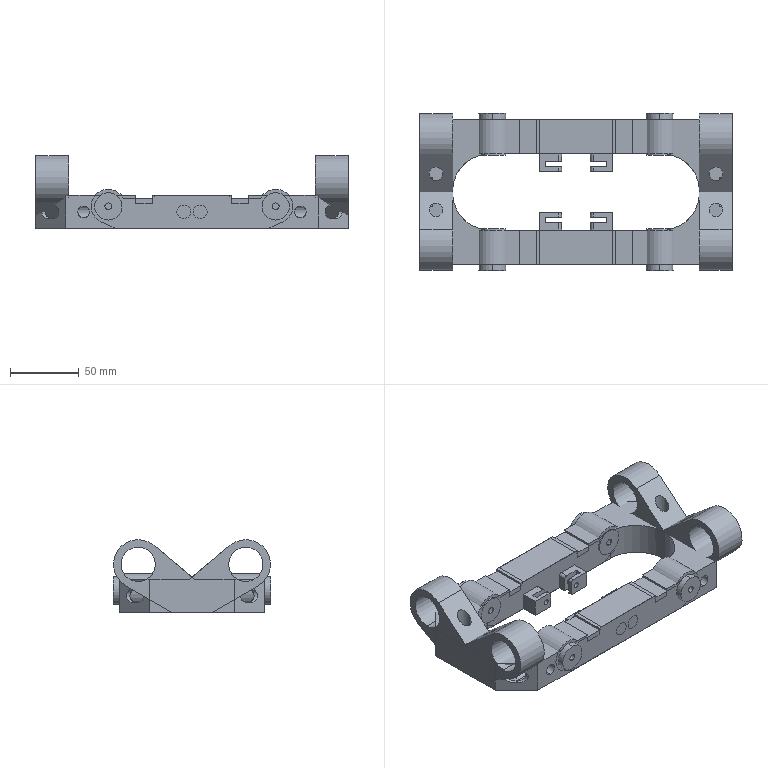NC program | Mastercam | posted with a generic post | part box 228 x 114.503 x 53 mm
Lines 3807 to 4701 of 27132:
(50 FEM |TOOL - 23|DIA. OFF. - 23|LEN. - 23|TOOL DIA. - 50.)
N7652 T23 M6
N7654 G0 G54 G90 X92.548 Y31.5 C0. B180. S5000 M3
N7656 G43 H23 Z278.
N7658 Z233.
N7660 G1 Z227.5 F600.
N7662 X87.548 F4000.
N7664 G3 X82.548 Y26.5 J-5.
N7666 G1 Y2.5
N7668 G2 X57.248 Y-22.8 I-25.3
N7670 G1 X11.069
N7672 X-11.419 Y-41.67
N7674 G2 X-39.252 Y-51.8 I-27.833 J33.17
N7676 X-82.552 Y-8.5 J43.3
N7678 X-60.902 Y28.999 I43.3
N7680 G1 X-21.409 Y51.8
N7682 X57.248
N7684 G2 X82.548 Y26.5 J-25.3
N7686 G1 Y21.5
N7688 G3 X87.548 Y16.5 I5.
N7690 G1 X92.548
N7692 Y31.5
N7694 Z227. F600.
N7696 X87.548 F4000.
N7698 G3 X82.548 Y26.5 J-5.
N7700 G1 Y2.5
N7702 G2 X57.248 Y-22.8 I-25.3
N7704 G1 X11.069
N7706 X-11.419 Y-41.67
N7708 G2 X-39.252 Y-51.8 I-27.833 J33.17
N7710 X-82.552 Y-8.5 J43.3
N7712 X-60.902 Y28.999 I43.3
N7714 G1 X-21.409 Y51.8
N7716 X57.248
N7718 G2 X82.548 Y26.5 J-25.3
N7720 G1 Y21.5
N7722 G3 X87.548 Y16.5 I5.
N7724 G1 X92.548
N7726 Y31.5
N7728 Z226.5 F600.
N7730 X87.548 F4000.
N7732 G3 X82.548 Y26.5 J-5.
N7734 G1 Y2.5
N7736 G2 X57.248 Y-22.8 I-25.3
N7738 G1 X11.069
N7740 X-11.419 Y-41.67
N7742 G2 X-39.252 Y-51.8 I-27.833 J33.17
N7744 X-82.552 Y-8.5 J43.3
N7746 X-60.902 Y28.999 I43.3
N7748 G1 X-21.409 Y51.8
N7750 X57.248
N7752 G2 X82.548 Y26.5 J-25.3
N7754 G1 Y21.5
N7756 G3 X87.548 Y16.5 I5.
N7758 G1 X92.548
N7760 Y31.5
N7762 Z226. F600.
N7764 X87.548 F4000.
N7766 G3 X82.548 Y26.5 J-5.
N7768 G1 Y2.5
N7770 G2 X57.248 Y-22.8 I-25.3
N7772 G1 X11.069
N7774 X-11.419 Y-41.67
N7776 G2 X-39.252 Y-51.8 I-27.833 J33.17
N7778 X-82.552 Y-8.5 J43.3
N7780 X-60.902 Y28.999 I43.3
N7782 G1 X-21.409 Y51.8
N7784 X57.248
N7786 G2 X82.548 Y26.5 J-25.3
N7788 G1 Y21.5
N7790 G3 X87.548 Y16.5 I5.
N7792 G1 X92.548
N7794 Y31.5
N7796 Z225.5 F600.
N7798 X87.548 F4000.
N7800 G3 X82.548 Y26.5 J-5.
N7802 G1 Y2.5
N7804 G2 X57.248 Y-22.8 I-25.3
N7806 G1 X11.069
N7808 X-11.419 Y-41.67
N7810 G2 X-39.252 Y-51.8 I-27.833 J33.17
N7812 X-82.552 Y-8.5 J43.3
N7814 X-60.902 Y28.999 I43.3
N7816 G1 X-21.409 Y51.8
N7818 X57.248
N7820 G2 X82.548 Y26.5 J-25.3
N7822 G1 Y21.5
N7824 G3 X87.548 Y16.5 I5.
N7826 G1 X92.548
N7828 Y31.5
N7830 Z225. F600.
N7832 X87.548 F4000.
N7834 G3 X82.548 Y26.5 J-5.
N7836 G1 Y2.5
N7838 G2 X57.248 Y-22.8 I-25.3
N7840 G1 X11.069
N7842 X-11.419 Y-41.67
N7844 G2 X-39.252 Y-51.8 I-27.833 J33.17
N7846 X-82.552 Y-8.5 J43.3
N7848 X-60.902 Y28.999 I43.3
N7850 G1 X-21.409 Y51.8
N7852 X57.248
N7854 G2 X82.548 Y26.5 J-25.3
N7856 G1 Y21.5
N7858 G3 X87.548 Y16.5 I5.
N7860 G1 X92.548
N7862 Y31.5
N7864 Z224.5 F600.
N7866 X87.548 F4000.
N7868 G3 X82.548 Y26.5 J-5.
N7870 G1 Y2.5
N7872 G2 X57.248 Y-22.8 I-25.3
N7874 G1 X11.069
N7876 X-11.419 Y-41.67
N7878 G2 X-39.252 Y-51.8 I-27.833 J33.17
N7880 X-82.552 Y-8.5 J43.3
N7882 X-60.902 Y28.999 I43.3
N7884 G1 X-21.409 Y51.8
N7886 X57.248
N7888 G2 X82.548 Y26.5 J-25.3
N7890 G1 Y21.5
N7892 G3 X87.548 Y16.5 I5.
N7894 G1 X92.548
N7896 Y31.5
N7898 Z224. F600.
N7900 X87.548 F4000.
N7902 G3 X82.548 Y26.5 J-5.
N7904 G1 Y2.5
N7906 G2 X57.248 Y-22.8 I-25.3
N7908 G1 X11.069
N7910 X-11.419 Y-41.67
N7912 G2 X-39.252 Y-51.8 I-27.833 J33.17
N7914 X-82.552 Y-8.5 J43.3
N7916 X-60.902 Y28.999 I43.3
N7918 G1 X-21.409 Y51.8
N7920 X57.248
N7922 G2 X82.548 Y26.5 J-25.3
N7924 G1 Y21.5
N7926 G3 X87.548 Y16.5 I5.
N7928 G1 X92.548
N7930 Y31.5
N7932 Z223.5 F600.
N7934 X87.548 F4000.
N7936 G3 X82.548 Y26.5 J-5.
N7938 G1 Y2.5
N7940 G2 X57.248 Y-22.8 I-25.3
N7942 G1 X11.069
N7944 X-11.419 Y-41.67
N7946 G2 X-39.252 Y-51.8 I-27.833 J33.17
N7948 X-82.552 Y-8.5 J43.3
N7950 X-60.902 Y28.999 I43.3
N7952 G1 X-21.409 Y51.8
N7954 X57.248
N7956 G2 X82.548 Y26.5 J-25.3
N7958 G1 Y21.5
N7960 G3 X87.548 Y16.5 I5.
N7962 G1 X92.548
N7964 Y31.5
N7966 Z223. F600.
N7968 X87.548 F4000.
N7970 G3 X82.548 Y26.5 J-5.
N7972 G1 Y2.5
N7974 G2 X57.248 Y-22.8 I-25.3
N7976 G1 X11.069
N7978 X-11.419 Y-41.67
N7980 G2 X-39.252 Y-51.8 I-27.833 J33.17
N7982 X-82.552 Y-8.5 J43.3
N7984 X-60.902 Y28.999 I43.3
N7986 G1 X-21.409 Y51.8
N7988 X57.248
N7990 G2 X82.548 Y26.5 J-25.3
N7992 G1 Y21.5
N7994 G3 X87.548 Y16.5 I5.
N7996 G1 X92.548
N7998 Y31.5
N8000 Z222.5 F600.
N8002 X87.548 F4000.
N8004 G3 X82.548 Y26.5 J-5.
N8006 G1 Y2.5
N8008 G2 X57.248 Y-22.8 I-25.3
N8010 G1 X11.069
N8012 X-11.419 Y-41.67
N8014 G2 X-39.252 Y-51.8 I-27.833 J33.17
N8016 X-82.552 Y-8.5 J43.3
N8018 X-60.902 Y28.999 I43.3
N8020 G1 X-21.409 Y51.8
N8022 X57.248
N8024 G2 X82.548 Y26.5 J-25.3
N8026 G1 Y21.5
N8028 G3 X87.548 Y16.5 I5.
N8030 G1 X92.548
N8032 Y31.5
N8034 Z222. F600.
N8036 X87.548 F4000.
N8038 G3 X82.548 Y26.5 J-5.
N8040 G1 Y2.5
N8042 G2 X57.248 Y-22.8 I-25.3
N8044 G1 X11.069
N8046 X-11.419 Y-41.67
N8048 G2 X-39.252 Y-51.8 I-27.833 J33.17
N8050 X-82.552 Y-8.5 J43.3
N8052 X-60.902 Y28.999 I43.3
N8054 G1 X-21.409 Y51.8
N8056 X57.248
N8058 G2 X82.548 Y26.5 J-25.3
N8060 G1 Y21.5
N8062 G3 X87.548 Y16.5 I5.
N8064 G1 X92.548
N8066 Y31.5
N8068 Z221.5 F600.
N8070 X87.548 F4000.
N8072 G3 X82.548 Y26.5 J-5.
N8074 G1 Y2.5
N8076 G2 X57.248 Y-22.8 I-25.3
N8078 G1 X11.069
N8080 X-11.419 Y-41.67
N8082 G2 X-39.252 Y-51.8 I-27.833 J33.17
N8084 X-82.552 Y-8.5 J43.3
N8086 X-60.902 Y28.999 I43.3
N8088 G1 X-21.409 Y51.8
N8090 X57.248
N8092 G2 X82.548 Y26.5 J-25.3
N8094 G1 Y21.5
N8096 G3 X87.548 Y16.5 I5.
N8098 G1 X92.548
N8100 Y31.5
N8102 Z221. F600.
N8104 X87.548 F4000.
N8106 G3 X82.548 Y26.5 J-5.
N8108 G1 Y2.5
N8110 G2 X57.248 Y-22.8 I-25.3
N8112 G1 X11.069
N8114 X-11.419 Y-41.67
N8116 G2 X-39.252 Y-51.8 I-27.833 J33.17
N8118 X-82.552 Y-8.5 J43.3
N8120 X-60.902 Y28.999 I43.3
N8122 G1 X-21.409 Y51.8
N8124 X57.248
N8126 G2 X82.548 Y26.5 J-25.3
N8128 G1 Y21.5
N8130 G3 X87.548 Y16.5 I5.
N8132 G1 X92.548
N8134 Y31.5
N8136 Z220.5 F600.
N8138 X87.548 F4000.
N8140 G3 X82.548 Y26.5 J-5.
N8142 G1 Y2.5
N8144 G2 X57.248 Y-22.8 I-25.3
N8146 G1 X11.069
N8148 X-11.419 Y-41.67
N8150 G2 X-39.252 Y-51.8 I-27.833 J33.17
N8152 X-82.552 Y-8.5 J43.3
N8154 X-60.902 Y28.999 I43.3
N8156 G1 X-21.409 Y51.8
N8158 X57.248
N8160 G2 X82.548 Y26.5 J-25.3
N8162 G1 Y21.5
N8164 G3 X87.548 Y16.5 I5.
N8166 G1 X92.548
N8168 Y31.5
N8170 Z220. F600.
N8172 X87.548 F4000.
N8174 G3 X82.548 Y26.5 J-5.
N8176 G1 Y2.5
N8178 G2 X57.248 Y-22.8 I-25.3
N8180 G1 X11.069
N8182 X-11.419 Y-41.67
N8184 G2 X-39.252 Y-51.8 I-27.833 J33.17
N8186 X-82.552 Y-8.5 J43.3
N8188 X-60.902 Y28.999 I43.3
N8190 G1 X-21.409 Y51.8
N8192 X57.248
N8194 G2 X82.548 Y26.5 J-25.3
N8196 G1 Y21.5
N8198 G3 X87.548 Y16.5 I5.
N8200 G1 X92.548
N8202 Y31.5
N8204 Z219.5 F600.
N8206 X87.548 F4000.
N8208 G3 X82.548 Y26.5 J-5.
N8210 G1 Y2.5
N8212 G2 X57.248 Y-22.8 I-25.3
N8214 G1 X11.069
N8216 X-11.419 Y-41.67
N8218 G2 X-39.252 Y-51.8 I-27.833 J33.17
N8220 X-82.552 Y-8.5 J43.3
N8222 X-60.902 Y28.999 I43.3
N8224 G1 X-21.409 Y51.8
N8226 X57.248
N8228 G2 X82.548 Y26.5 J-25.3
N8230 G1 Y21.5
N8232 G3 X87.548 Y16.5 I5.
N8234 G1 X92.548
N8236 Y31.5
N8238 Z219. F600.
N8240 X87.548 F4000.
N8242 G3 X82.548 Y26.5 J-5.
N8244 G1 Y2.5
N8246 G2 X57.248 Y-22.8 I-25.3
N8248 G1 X11.069
N8250 X-11.419 Y-41.67
N8252 G2 X-39.252 Y-51.8 I-27.833 J33.17
N8254 X-82.552 Y-8.5 J43.3
N8256 X-60.902 Y28.999 I43.3
N8258 G1 X-21.409 Y51.8
N8260 X57.248
N8262 G2 X82.548 Y26.5 J-25.3
N8264 G1 Y21.5
N8266 G3 X87.548 Y16.5 I5.
N8268 G1 X92.548
N8270 Y31.5
N8272 Z218.5 F600.
N8274 X87.548 F4000.
N8276 G3 X82.548 Y26.5 J-5.
N8278 G1 Y2.5
N8280 G2 X57.248 Y-22.8 I-25.3
N8282 G1 X11.069
N8284 X-11.419 Y-41.67
N8286 G2 X-39.252 Y-51.8 I-27.833 J33.17
N8288 X-82.552 Y-8.5 J43.3
N8290 X-60.902 Y28.999 I43.3
N8292 G1 X-21.409 Y51.8
N8294 X57.248
N8296 G2 X82.548 Y26.5 J-25.3
N8298 G1 Y21.5
N8300 G3 X87.548 Y16.5 I5.
N8302 G1 X92.548
N8304 Y31.5
N8306 Z218. F600.
N8308 X87.548 F4000.
N8310 G3 X82.548 Y26.5 J-5.
N8312 G1 Y2.5
N8314 G2 X57.248 Y-22.8 I-25.3
N8316 G1 X11.069
N8318 X-11.419 Y-41.67
N8320 G2 X-39.252 Y-51.8 I-27.833 J33.17
N8322 X-82.552 Y-8.5 J43.3
N8324 X-60.902 Y28.999 I43.3
N8326 G1 X-21.409 Y51.8
N8328 X57.248
N8330 G2 X82.548 Y26.5 J-25.3
N8332 G1 Y21.5
N8334 G3 X87.548 Y16.5 I5.
N8336 G1 X92.548
N8338 Y31.5
N8340 Z217.5 F600.
N8342 X87.548 F4000.
N8344 G3 X82.548 Y26.5 J-5.
N8346 G1 Y2.5
N8348 G2 X57.248 Y-22.8 I-25.3
N8350 G1 X11.069
N8352 X-11.419 Y-41.67
N8354 G2 X-39.252 Y-51.8 I-27.833 J33.17
N8356 X-82.552 Y-8.5 J43.3
N8358 X-60.902 Y28.999 I43.3
N8360 G1 X-21.409 Y51.8
N8362 X57.248
N8364 G2 X82.548 Y26.5 J-25.3
N8366 G1 Y21.5
N8368 G3 X87.548 Y16.5 I5.
N8370 G1 X92.548
N8372 Y31.5
N8374 Z217. F600.
N8376 X87.548 F4000.
N8378 G3 X82.548 Y26.5 J-5.
N8380 G1 Y2.5
N8382 G2 X57.248 Y-22.8 I-25.3
N8384 G1 X11.069
N8386 X-11.419 Y-41.67
N8388 G2 X-39.252 Y-51.8 I-27.833 J33.17
N8390 X-82.552 Y-8.5 J43.3
N8392 X-60.902 Y28.999 I43.3
N8394 G1 X-21.409 Y51.8
N8396 X57.248
N8398 G2 X82.548 Y26.5 J-25.3
N8400 G1 Y21.5
N8402 G3 X87.548 Y16.5 I5.
N8404 G1 X92.548
N8406 Y31.5
N8408 Z216.5 F600.
N8410 X87.548 F4000.
N8412 G3 X82.548 Y26.5 J-5.
N8414 G1 Y2.5
N8416 G2 X57.248 Y-22.8 I-25.3
N8418 G1 X11.069
N8420 X-11.419 Y-41.67
N8422 G2 X-39.252 Y-51.8 I-27.833 J33.17
N8424 X-82.552 Y-8.5 J43.3
N8426 X-60.902 Y28.999 I43.3
N8428 G1 X-21.409 Y51.8
N8430 X57.248
N8432 G2 X82.548 Y26.5 J-25.3
N8434 G1 Y21.5
N8436 G3 X87.548 Y16.5 I5.
N8438 G1 X92.548
N8440 Y31.5
N8442 Z216. F600.
N8444 X87.548 F4000.
N8446 G3 X82.548 Y26.5 J-5.
N8448 G1 Y2.5
N8450 G2 X57.248 Y-22.8 I-25.3
N8452 G1 X11.069
N8454 X-11.419 Y-41.67
N8456 G2 X-39.252 Y-51.8 I-27.833 J33.17
N8458 X-82.552 Y-8.5 J43.3
N8460 X-60.902 Y28.999 I43.3
N8462 G1 X-21.409 Y51.8
N8464 X57.248
N8466 G2 X82.548 Y26.5 J-25.3
N8468 G1 Y21.5
N8470 G3 X87.548 Y16.5 I5.
N8472 G1 X92.548
N8474 Y31.5
N8476 Z215.5 F600.
N8478 X87.548 F4000.
N8480 G3 X82.548 Y26.5 J-5.
N8482 G1 Y2.5
N8484 G2 X57.248 Y-22.8 I-25.3
N8486 G1 X11.069
N8488 X-11.419 Y-41.67
N8490 G2 X-39.252 Y-51.8 I-27.833 J33.17
N8492 X-82.552 Y-8.5 J43.3
N8494 X-60.902 Y28.999 I43.3
N8496 G1 X-21.409 Y51.8
N8498 X57.248
N8500 G2 X82.548 Y26.5 J-25.3
N8502 G1 Y21.5
N8504 G3 X87.548 Y16.5 I5.
N8506 G1 X92.548
N8508 Y31.5
N8510 Z215. F600.
N8512 X87.548 F4000.
N8514 G3 X82.548 Y26.5 J-5.
N8516 G1 Y2.5
N8518 G2 X57.248 Y-22.8 I-25.3
N8520 G1 X11.069
N8522 X-11.419 Y-41.67
N8524 G2 X-39.252 Y-51.8 I-27.833 J33.17
N8526 X-82.552 Y-8.5 J43.3
N8528 X-60.902 Y28.999 I43.3
N8530 G1 X-21.409 Y51.8
N8532 X57.248
N8534 G2 X82.548 Y26.5 J-25.3
N8536 G1 Y21.5
N8538 G3 X87.548 Y16.5 I5.
N8540 G1 X92.548
N8542 Y31.5
N8544 Z214.5 F600.
N8546 X87.548 F4000.
N8548 G3 X82.548 Y26.5 J-5.
N8550 G1 Y2.5
N8552 G2 X57.248 Y-22.8 I-25.3
N8554 G1 X11.069
N8556 X-11.419 Y-41.67
N8558 G2 X-39.252 Y-51.8 I-27.833 J33.17
N8560 X-82.552 Y-8.5 J43.3
N8562 X-60.902 Y28.999 I43.3
N8564 G1 X-21.409 Y51.8
N8566 X57.248
N8568 G2 X82.548 Y26.5 J-25.3
N8570 G1 Y21.5
N8572 G3 X87.548 Y16.5 I5.
N8574 G1 X92.548
N8576 Y31.5
N8578 Z214. F600.
N8580 X87.548 F4000.
N8582 G3 X82.548 Y26.5 J-5.
N8584 G1 Y2.5
N8586 G2 X57.248 Y-22.8 I-25.3
N8588 G1 X11.069
N8590 X-11.419 Y-41.67
N8592 G2 X-39.252 Y-51.8 I-27.833 J33.17
N8594 X-82.552 Y-8.5 J43.3
N8596 X-60.902 Y28.999 I43.3
N8598 G1 X-21.409 Y51.8
N8600 X57.248
N8602 G2 X82.548 Y26.5 J-25.3
N8604 G1 Y21.5
N8606 G3 X87.548 Y16.5 I5.
N8608 G1 X92.548
N8610 Y31.5
N8612 Z213.5 F600.
N8614 X87.548 F4000.
N8616 G3 X82.548 Y26.5 J-5.
N8618 G1 Y2.5
N8620 G2 X57.248 Y-22.8 I-25.3
N8622 G1 X11.069
N8624 X-11.419 Y-41.67
N8626 G2 X-39.252 Y-51.8 I-27.833 J33.17
N8628 X-82.552 Y-8.5 J43.3
N8630 X-60.902 Y28.999 I43.3
N8632 G1 X-21.409 Y51.8
N8634 X57.248
N8636 G2 X82.548 Y26.5 J-25.3
N8638 G1 Y21.5
N8640 G3 X87.548 Y16.5 I5.
N8642 G1 X92.548
N8644 Y31.5
N8646 Z213. F600.
N8648 X87.548 F4000.
N8650 G3 X82.548 Y26.5 J-5.
N8652 G1 Y2.5
N8654 G2 X57.248 Y-22.8 I-25.3
N8656 G1 X11.069
N8658 X-11.419 Y-41.67
N8660 G2 X-39.252 Y-51.8 I-27.833 J33.17
N8662 X-82.552 Y-8.5 J43.3
N8664 X-60.902 Y28.999 I43.3
N8666 G1 X-21.409 Y51.8
N8668 X57.248
N8670 G2 X82.548 Y26.5 J-25.3
N8672 G1 Y21.5
N8674 G3 X87.548 Y16.5 I5.
N8676 G1 X92.548
N8678 Y31.5
N8680 Z212.5 F600.
N8682 X87.548 F4000.
N8684 G3 X82.548 Y26.5 J-5.
N8686 G1 Y2.5
N8688 G2 X57.248 Y-22.8 I-25.3
N8690 G1 X11.069
N8692 X-11.419 Y-41.67
N8694 G2 X-39.252 Y-51.8 I-27.833 J33.17
N8696 X-82.552 Y-8.5 J43.3
N8698 X-60.902 Y28.999 I43.3
N8700 G1 X-21.409 Y51.8
N8702 X57.248
N8704 G2 X82.548 Y26.5 J-25.3
N8706 G1 Y21.5
N8708 G3 X87.548 Y16.5 I5.
N8710 G1 X92.548
N8712 Y31.5
N8714 Z212. F600.
N8716 X87.548 F4000.
N8718 G3 X82.548 Y26.5 J-5.
N8720 G1 Y2.5
N8722 G2 X57.248 Y-22.8 I-25.3
N8724 G1 X11.069
N8726 X-11.419 Y-41.67
N8728 G2 X-39.252 Y-51.8 I-27.833 J33.17
N8730 X-82.552 Y-8.5 J43.3
N8732 X-60.902 Y28.999 I43.3
N8734 G1 X-21.409 Y51.8
N8736 X57.248
N8738 G2 X82.548 Y26.5 J-25.3
N8740 G1 Y21.5
N8742 G3 X87.548 Y16.5 I5.
N8744 G1 X92.548
N8746 Y31.5
N8748 Z211.5 F600.
N8750 X87.548 F4000.
N8752 G3 X82.548 Y26.5 J-5.
N8754 G1 Y2.5
N8756 G2 X57.248 Y-22.8 I-25.3
N8758 G1 X11.069
N8760 X-11.419 Y-41.67
N8762 G2 X-39.252 Y-51.8 I-27.833 J33.17
N8764 X-82.552 Y-8.5 J43.3
N8766 X-60.902 Y28.999 I43.3
N8768 G1 X-21.409 Y51.8
N8770 X57.248
N8772 G2 X82.548 Y26.5 J-25.3
N8774 G1 Y21.5
N8776 G3 X87.548 Y16.5 I5.
N8778 G1 X92.548
N8780 Y31.5
N8782 Z211. F600.
N8784 X87.548 F4000.
N8786 G3 X82.548 Y26.5 J-5.
N8788 G1 Y2.5
N8790 G2 X57.248 Y-22.8 I-25.3
N8792 G1 X11.069
N8794 X-11.419 Y-41.67
N8796 G2 X-39.252 Y-51.8 I-27.833 J33.17
N8798 X-82.552 Y-8.5 J43.3
N8800 X-60.902 Y28.999 I43.3
N8802 G1 X-21.409 Y51.8
N8804 X57.248
N8806 G2 X82.548 Y26.5 J-25.3
N8808 G1 Y21.5
N8810 G3 X87.548 Y16.5 I5.
N8812 G1 X92.548
N8814 Y31.5
N8816 Z210.5 F600.
N8818 X87.548 F4000.
N8820 G3 X82.548 Y26.5 J-5.
N8822 G1 Y2.5
N8824 G2 X57.248 Y-22.8 I-25.3
N8826 G1 X11.069
N8828 X-11.419 Y-41.67
N8830 G2 X-39.252 Y-51.8 I-27.833 J33.17
N8832 X-82.552 Y-8.5 J43.3
N8834 X-60.902 Y28.999 I43.3
N8836 G1 X-21.409 Y51.8
N8838 X57.248
N8840 G2 X82.548 Y26.5 J-25.3
N8842 G1 Y21.5
N8844 G3 X87.548 Y16.5 I5.
N8846 G1 X92.548
N8848 Y31.5
N8850 Z210. F600.
N8852 X87.548 F4000.
N8854 G3 X82.548 Y26.5 J-5.
N8856 G1 Y2.5
N8858 G2 X57.248 Y-22.8 I-25.3
N8860 G1 X11.069
N8862 X-11.419 Y-41.67
N8864 G2 X-39.252 Y-51.8 I-27.833 J33.17
N8866 X-82.552 Y-8.5 J43.3
N8868 X-60.902 Y28.999 I43.3
N8870 G1 X-21.409 Y51.8
N8872 X57.248
N8874 G2 X82.548 Y26.5 J-25.3
N8876 G1 Y21.5
N8878 G3 X87.548 Y16.5 I5.
N8880 G1 X92.548
N8882 Y31.5
N8884 Z209.5 F600.
N8886 X87.548 F4000.
N8888 G3 X82.548 Y26.5 J-5.
N8890 G1 Y2.5
N8892 G2 X57.248 Y-22.8 I-25.3
N8894 G1 X11.069
N8896 X-11.419 Y-41.67
N8898 G2 X-39.252 Y-51.8 I-27.833 J33.17
N8900 X-82.552 Y-8.5 J43.3
N8902 X-60.902 Y28.999 I43.3
N8904 G1 X-21.409 Y51.8
N8906 X57.248
N8908 G2 X82.548 Y26.5 J-25.3
N8910 G1 Y21.5
N8912 G3 X87.548 Y16.5 I5.
N8914 G1 X92.548
N8916 Y31.5
N8918 Z209. F600.
N8920 X87.548 F4000.
N8922 G3 X82.548 Y26.5 J-5.
N8924 G1 Y2.5
N8926 G2 X57.248 Y-22.8 I-25.3
N8928 G1 X11.069
N8930 X-11.419 Y-41.67
N8932 G2 X-39.252 Y-51.8 I-27.833 J33.17
N8934 X-82.552 Y-8.5 J43.3
N8936 X-60.902 Y28.999 I43.3
N8938 G1 X-21.409 Y51.8
N8940 X57.248
N8942 G2 X82.548 Y26.5 J-25.3
N8944 G1 Y21.5
N8946 G3 X87.548 Y16.5 I5.
N8948 G1 X92.548
N8950 Y31.5
N8952 Z208.5 F600.
N8954 X87.548 F4000.
N8956 G3 X82.548 Y26.5 J-5.
N8958 G1 Y2.5
N8960 G2 X57.248 Y-22.8 I-25.3
N8962 G1 X11.069
N8964 X-11.419 Y-41.67
N8966 G2 X-39.252 Y-51.8 I-27.833 J33.17
N8968 X-82.552 Y-8.5 J43.3
N8970 X-60.902 Y28.999 I43.3
N8972 G1 X-21.409 Y51.8
N8974 X57.248
N8976 G2 X82.548 Y26.5 J-25.3
N8978 G1 Y21.5
N8980 G3 X87.548 Y16.5 I5.
N8982 G1 X92.548
N8984 Y31.5
N8986 Z208. F600.
N8988 X87.548 F4000.
N8990 G3 X82.548 Y26.5 J-5.
N8992 G1 Y2.5
N8994 G2 X57.248 Y-22.8 I-25.3
N8996 G1 X11.069
N8998 X-11.419 Y-41.67
N9000 G2 X-39.252 Y-51.8 I-27.833 J33.17
N9002 X-82.552 Y-8.5 J43.3
N9004 X-60.902 Y28.999 I43.3
N9006 G1 X-21.409 Y51.8
N9008 X57.248
N9010 G2 X82.548 Y26.5 J-25.3
N9012 G1 Y21.5
N9014 G3 X87.548 Y16.5 I5.
N9016 G1 X92.548
N9018 Y31.5
N9020 Z207.5 F600.
N9022 X87.548 F4000.
N9024 G3 X82.548 Y26.5 J-5.
N9026 G1 Y2.5
N9028 G2 X57.248 Y-22.8 I-25.3
N9030 G1 X11.069
N9032 X-11.419 Y-41.67
N9034 G2 X-39.252 Y-51.8 I-27.833 J33.17
N9036 X-82.552 Y-8.5 J43.3
N9038 X-60.902 Y28.999 I43.3
N9040 G1 X-21.409 Y51.8
N9042 X57.248
N9044 G2 X82.548 Y26.5 J-25.3
N9046 G1 Y21.5
N9048 G3 X87.548 Y16.5 I5.
N9050 G1 X92.548
N9052 Y31.5
N9054 Z207. F600.
N9056 X87.548 F4000.
N9058 G3 X82.548 Y26.5 J-5.
N9060 G1 Y2.5
N9062 G2 X57.248 Y-22.8 I-25.3
N9064 G1 X11.069
N9066 X-11.419 Y-41.67
N9068 G2 X-39.252 Y-51.8 I-27.833 J33.17
N9070 X-82.552 Y-8.5 J43.3
N9072 X-60.902 Y28.999 I43.3
N9074 G1 X-21.409 Y51.8
N9076 X57.248
N9078 G2 X82.548 Y26.5 J-25.3
N9080 G1 Y21.5
N9082 G3 X87.548 Y16.5 I5.
N9084 G1 X92.548
N9086 Y31.5
N9088 Z206.5 F600.
N9090 X87.548 F4000.
N9092 G3 X82.548 Y26.5 J-5.
N9094 G1 Y2.5
N9096 G2 X57.248 Y-22.8 I-25.3
N9098 G1 X11.069
N9100 X-11.419 Y-41.67
N9102 G2 X-39.252 Y-51.8 I-27.833 J33.17
N9104 X-82.552 Y-8.5 J43.3
N9106 X-60.902 Y28.999 I43.3
N9108 G1 X-21.409 Y51.8
N9110 X57.248
N9112 G2 X82.548 Y26.5 J-25.3
N9114 G1 Y21.5
N9116 G3 X87.548 Y16.5 I5.
N9118 G1 X92.548
N9120 Y31.5
N9122 Z206. F600.
N9124 X87.548 F4000.
N9126 G3 X82.548 Y26.5 J-5.
N9128 G1 Y2.5
N9130 G2 X57.248 Y-22.8 I-25.3
N9132 G1 X11.069
N9134 X-11.419 Y-41.67
N9136 G2 X-39.252 Y-51.8 I-27.833 J33.17
N9138 X-82.552 Y-8.5 J43.3
N9140 X-60.902 Y28.999 I43.3
N9142 G1 X-21.409 Y51.8
N9144 X57.248
N9146 G2 X82.548 Y26.5 J-25.3
N9148 G1 Y21.5
N9150 G3 X87.548 Y16.5 I5.
N9152 G1 X92.548
N9154 Y31.5
N9156 Z205.5 F600.
N9158 X87.548 F4000.
N9160 G3 X82.548 Y26.5 J-5.
N9162 G1 Y2.5
N9164 G2 X57.248 Y-22.8 I-25.3
N9166 G1 X11.069
N9168 X-11.419 Y-41.67
N9170 G2 X-39.252 Y-51.8 I-27.833 J33.17
N9172 X-82.552 Y-8.5 J43.3
N9174 X-60.902 Y28.999 I43.3
N9176 G1 X-21.409 Y51.8
N9178 X57.248
N9180 G2 X82.548 Y26.5 J-25.3
N9182 G1 Y21.5
N9184 G3 X87.548 Y16.5 I5.
N9186 G1 X92.548
N9188 Y31.5
N9190 Z205. F600.
N9192 X87.548 F4000.
N9194 G3 X82.548 Y26.5 J-5.
N9196 G1 Y2.5
N9198 G2 X57.248 Y-22.8 I-25.3
N9200 G1 X11.069
N9202 X-11.419 Y-41.67
N9204 G2 X-39.252 Y-51.8 I-27.833 J33.17
N9206 X-82.552 Y-8.5 J43.3
N9208 X-60.902 Y28.999 I43.3
N9210 G1 X-21.409 Y51.8
N9212 X57.248
N9214 G2 X82.548 Y26.5 J-25.3
N9216 G1 Y21.5
N9218 G3 X87.548 Y16.5 I5.
N9220 G1 X92.548
N9222 Y31.5
N9224 Z204.5 F600.
N9226 X87.548 F4000.
N9228 G3 X82.548 Y26.5 J-5.
N9230 G1 Y2.5
N9232 G2 X57.248 Y-22.8 I-25.3
N9234 G1 X11.069
N9236 X-11.419 Y-41.67
N9238 G2 X-39.252 Y-51.8 I-27.833 J33.17
N9240 X-82.552 Y-8.5 J43.3
N9242 X-60.902 Y28.999 I43.3
N9244 G1 X-21.409 Y51.8
N9246 X57.248
N9248 G2 X82.548 Y26.5 J-25.3
N9250 G1 Y21.5
N9252 G3 X87.548 Y16.5 I5.
N9254 G1 X92.548
N9256 Y31.5
N9258 Z204. F600.
N9260 X87.548 F4000.
N9262 G3 X82.548 Y26.5 J-5.
N9264 G1 Y2.5
N9266 G2 X57.248 Y-22.8 I-25.3
N9268 G1 X11.069
N9270 X-11.419 Y-41.67
N9272 G2 X-39.252 Y-51.8 I-27.833 J33.17
N9274 X-82.552 Y-8.5 J43.3
N9276 X-60.902 Y28.999 I43.3
N9278 G1 X-21.409 Y51.8
N9280 X57.248
N9282 G2 X82.548 Y26.5 J-25.3
N9284 G1 Y21.5
N9286 G3 X87.548 Y16.5 I5.
N9288 G1 X92.548
N9290 Y31.5
N9292 Z203.5 F600.
N9294 X87.548 F4000.
N9296 G3 X82.548 Y26.5 J-5.
N9298 G1 Y2.5
N9300 G2 X57.248 Y-22.8 I-25.3
N9302 G1 X11.069
N9304 X-11.419 Y-41.67
N9306 G2 X-39.252 Y-51.8 I-27.833 J33.17
N9308 X-82.552 Y-8.5 J43.3
N9310 X-60.902 Y28.999 I43.3
N9312 G1 X-21.409 Y51.8
N9314 X57.248
N9316 G2 X82.548 Y26.5 J-25.3
N9318 G1 Y21.5
N9320 G3 X87.548 Y16.5 I5.
N9322 G1 X92.548
N9324 Y31.5
N9326 Z203. F600.
N9328 X87.548 F4000.
N9330 G3 X82.548 Y26.5 J-5.
N9332 G1 Y2.5
N9334 G2 X57.248 Y-22.8 I-25.3
N9336 G1 X11.069
N9338 X-11.419 Y-41.67
N9340 G2 X-39.252 Y-51.8 I-27.833 J33.17
N9342 X-82.552 Y-8.5 J43.3
N9344 X-60.902 Y28.999 I43.3
N9346 G1 X-21.409 Y51.8
N9348 X57.248
N9350 G2 X82.548 Y26.5 J-25.3
N9352 G1 Y21.5
N9354 G3 X87.548 Y16.5 I5.
N9356 G1 X92.548
N9358 Y31.5
N9360 Z202.5 F600.
N9362 X87.548 F4000.
N9364 G3 X82.548 Y26.5 J-5.
N9366 G1 Y2.5
N9368 G2 X57.248 Y-22.8 I-25.3
N9370 G1 X11.069
N9372 X-11.419 Y-41.67
N9374 G2 X-39.252 Y-51.8 I-27.833 J33.17
N9376 X-82.552 Y-8.5 J43.3
N9378 X-60.902 Y28.999 I43.3
N9380 G1 X-21.409 Y51.8
N9382 X57.248
N9384 G2 X82.548 Y26.5 J-25.3
N9386 G1 Y21.5
N9388 G3 X87.548 Y16.5 I5.
N9390 G1 X92.548
N9392 Y31.5
N9394 Z202. F600.
N9396 X87.548 F4000.
N9398 G3 X82.548 Y26.5 J-5.
N9400 G1 Y2.5
N9402 G2 X57.248 Y-22.8 I-25.3
N9404 G1 X11.069
N9406 X-11.419 Y-41.67
N9408 G2 X-39.252 Y-51.8 I-27.833 J33.17
N9410 X-82.552 Y-8.5 J43.3
N9412 X-60.902 Y28.999 I43.3
N9414 G1 X-21.409 Y51.8
N9416 X57.248
N9418 G2 X82.548 Y26.5 J-25.3
N9420 G1 Y21.5
N9422 G3 X87.548 Y16.5 I5.
N9424 G1 X92.548
N9426 G0 Z278.
N9428 M5
N9430 G0 G28 G91 Z0.
N9432 G28 B0.
N9434 M01
N9436 G0 G17 G40 G80 G90 G94 G98
N9438 G0 G28 G91 Z0.